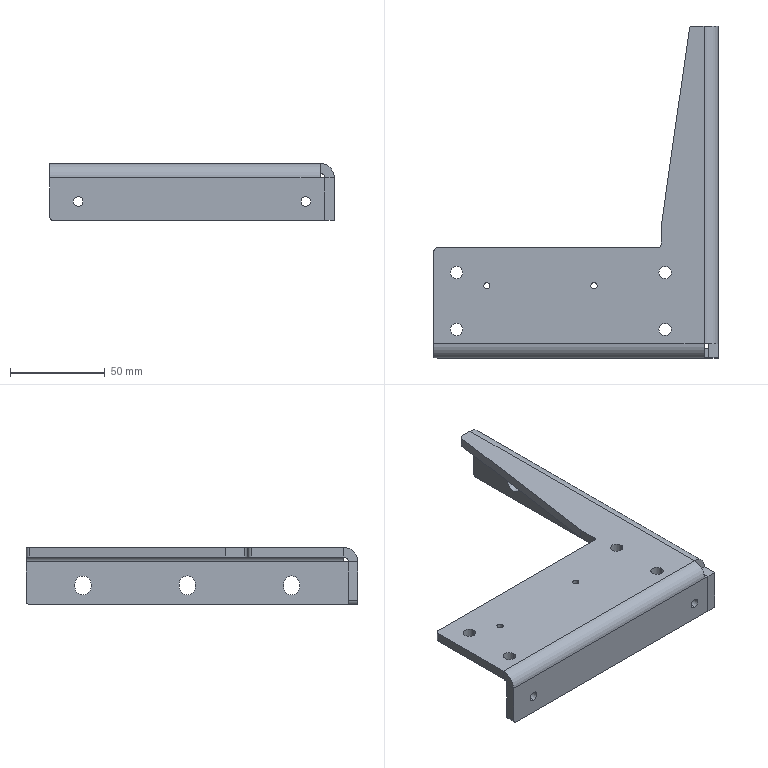Part | STEP file | Right-angle fixing plate A | 1 solid | 63 faces | box 150 x 175 x 30 mm | volume 91369 mm3 | cylinder 34 | plane 29 | commonest cylinder face diameters 8.5 x9 6.5 x8 5 x6 4 x5 3.3 x4 15 x2